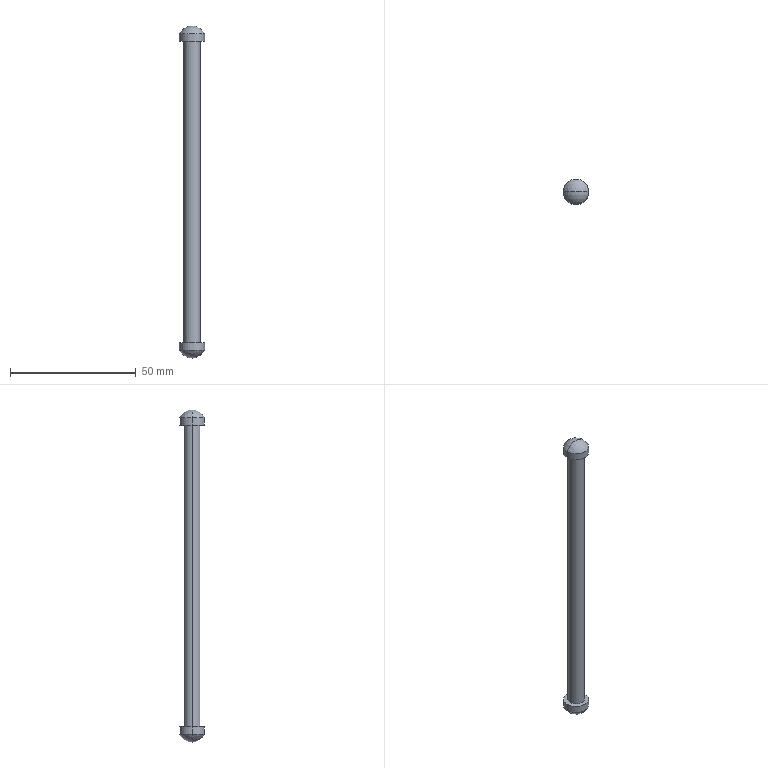Part | SolidWorks | features BaseBody 1 | 1 solid | 12 faces | box 10 x 10 x 132 mm | volume 4717 mm3 | cylinder 6 | sphere 4 | plane 2 | commonest cylinder face diameters 10 x4 6.5 x2
STEP:
#1=CARTESIAN_POINT('',(-30.,5.,-126.));
#2=VERTEX_POINT('',#1);
#3=CARTESIAN_POINT('',(-25.,5.,-123.));
#4=VERTEX_POINT('',#3);
#5=CARTESIAN_POINT('',(-30.,5.,-120.333));
#6=DIRECTION('',(0.,-1.,0.));
#7=DIRECTION('',(0.,0.,-1.));
#8=AXIS2_PLACEMENT_3D('',#5,#6,#7);
#9=CIRCLE('',#8,5.667);
#10=EDGE_CURVE('',#2,#4,#9,.T.);
#11=ORIENTED_EDGE('',*,*,#10,.F.);
#12=CARTESIAN_POINT('',(-35.,5.,-123.));
#13=VERTEX_POINT('',#12);
#14=CARTESIAN_POINT('',(-30.,5.,-120.333));
#15=DIRECTION('',(0.,1.,0.));
#16=DIRECTION('',(-1.,0.,0.));
#17=AXIS2_PLACEMENT_3D('',#14,#15,#16);
#18=CIRCLE('',#17,5.667);
#19=EDGE_CURVE('',#2,#13,#18,.T.);
#20=ORIENTED_EDGE('',*,*,#19,.T.);
#21=CARTESIAN_POINT('',(-30.,5.,-123.));
#22=DIRECTION('',(0.,0.,1.));
#23=DIRECTION('',(1.,0.,0.));
#24=AXIS2_PLACEMENT_3D('',#21,#22,#23);
#25=CIRCLE('',#24,5.);
#26=EDGE_CURVE('',#4,#13,#25,.T.);
#27=ORIENTED_EDGE('',*,*,#26,.F.);
#28=EDGE_LOOP('',(#11,#20,#27));
#29=FACE_OUTER_BOUND('',#28,.T.);
#30=CARTESIAN_POINT('',(-30.,5.,-120.333));
#31=DIRECTION('',(0.,1.,0.));
#32=DIRECTION('',(1.,0.,0.));
#33=AXIS2_PLACEMENT_3D('',#30,#31,#32);
#34=SPHERICAL_SURFACE('',#33,5.667);
#35=ADVANCED_FACE('',(#29),#34,.T.);
#36=ORIENTED_EDGE('',*,*,#26,.T.);
#37=CARTESIAN_POINT('',(-35.,5.,-120.));
#38=VERTEX_POINT('',#37);
#39=CARTESIAN_POINT('',(-35.,5.,-123.));
#40=DIRECTION('',(0.,0.,1.));
#41=VECTOR('',#40,1000.);
#42=LINE('',#39,#41);
#43=EDGE_CURVE('',#13,#38,#42,.T.);
#44=ORIENTED_EDGE('',*,*,#43,.T.);
#45=CARTESIAN_POINT('',(-25.,5.,-120.));
#46=VERTEX_POINT('',#45);
#47=CARTESIAN_POINT('',(-30.,5.,-120.));
#48=DIRECTION('',(0.,0.,1.));
#49=DIRECTION('',(1.,0.,0.));
#50=AXIS2_PLACEMENT_3D('',#47,#48,#49);
#51=CIRCLE('',#50,5.);
#52=EDGE_CURVE('',#46,#38,#51,.T.);
#53=ORIENTED_EDGE('',*,*,#52,.F.);
#54=CARTESIAN_POINT('',(-25.,5.,-123.));
#55=DIRECTION('',(0.,0.,1.));
#56=VECTOR('',#55,1000.);
#57=LINE('',#54,#56);
#58=EDGE_CURVE('',#4,#46,#57,.T.);
#59=ORIENTED_EDGE('',*,*,#58,.F.);
#60=EDGE_LOOP('',(#36,#44,#53,#59));
#61=FACE_OUTER_BOUND('',#60,.T.);
#62=CARTESIAN_POINT('',(-30.,5.,-123.));
#63=DIRECTION('',(0.,0.,1.));
#64=DIRECTION('',(1.,0.,0.));
#65=AXIS2_PLACEMENT_3D('',#62,#63,#64);
#66=CYLINDRICAL_SURFACE('',#65,5.);
#67=ADVANCED_FACE('',(#61),#66,.T.);
#68=CARTESIAN_POINT('',(-25.,5.,3.));
#69=VERTEX_POINT('',#68);
#70=CARTESIAN_POINT('',(-35.,5.,3.));
#71=VERTEX_POINT('',#70);
#72=CARTESIAN_POINT('',(-30.,5.,3.));
#73=DIRECTION('',(0.,0.,1.));
#74=DIRECTION('',(1.,0.,0.));
#75=AXIS2_PLACEMENT_3D('',#72,#73,#74);
#76=CIRCLE('',#75,5.);
#77=EDGE_CURVE('',#69,#71,#76,.T.);
#78=ORIENTED_EDGE('',*,*,#77,.T.);
#79=CARTESIAN_POINT('',(-30.,5.,6.));
#80=VERTEX_POINT('',#79);
#81=CARTESIAN_POINT('',(-30.,5.,0.3333));
#82=DIRECTION('',(0.,1.,0.));
#83=DIRECTION('',(-1.,0.,0.));
#84=AXIS2_PLACEMENT_3D('',#81,#82,#83);
#85=CIRCLE('',#84,5.667);
#86=EDGE_CURVE('',#71,#80,#85,.T.);
#87=ORIENTED_EDGE('',*,*,#86,.T.);
#88=CARTESIAN_POINT('',(-30.,5.,0.3333));
#89=DIRECTION('',(0.,-1.,0.));
#90=DIRECTION('',(0.,0.,-1.));
#91=AXIS2_PLACEMENT_3D('',#88,#89,#90);
#92=CIRCLE('',#91,5.667);
#93=EDGE_CURVE('',#69,#80,#92,.T.);
#94=ORIENTED_EDGE('',*,*,#93,.F.);
#95=EDGE_LOOP('',(#78,#87,#94));
#96=FACE_OUTER_BOUND('',#95,.T.);
#97=CARTESIAN_POINT('',(-30.,5.,0.3333));
#98=DIRECTION('',(0.,1.,0.));
#99=DIRECTION('',(1.,0.,0.));
#100=AXIS2_PLACEMENT_3D('',#97,#98,#99);
#101=SPHERICAL_SURFACE('',#100,5.667);
#102=ADVANCED_FACE('',(#96),#101,.T.);
#103=ORIENTED_EDGE('',*,*,#77,.F.);
#104=CARTESIAN_POINT('',(-25.,5.,0.));
#105=VERTEX_POINT('',#104);
#106=CARTESIAN_POINT('',(-25.,5.,3.));
#107=DIRECTION('',(0.,0.,-1.));
#108=VECTOR('',#107,1000.);
#109=LINE('',#106,#108);
#110=EDGE_CURVE('',#69,#105,#109,.T.);
#111=ORIENTED_EDGE('',*,*,#110,.T.);
#112=CARTESIAN_POINT('',(-35.,5.,0.));
#113=VERTEX_POINT('',#112);
#114=CARTESIAN_POINT('',(-30.,5.,0.));
#115=DIRECTION('',(0.,0.,1.));
#116=DIRECTION('',(1.,0.,0.));
#117=AXIS2_PLACEMENT_3D('',#114,#115,#116);
#118=CIRCLE('',#117,5.);
#119=EDGE_CURVE('',#105,#113,#118,.T.);
#120=ORIENTED_EDGE('',*,*,#119,.T.);
#121=CARTESIAN_POINT('',(-35.,5.,3.));
#122=DIRECTION('',(0.,0.,-1.));
#123=VECTOR('',#122,1000.);
#124=LINE('',#121,#123);
#125=EDGE_CURVE('',#71,#113,#124,.T.);
#126=ORIENTED_EDGE('',*,*,#125,.F.);
#127=EDGE_LOOP('',(#103,#111,#120,#126));
#128=FACE_OUTER_BOUND('',#127,.T.);
#129=CARTESIAN_POINT('',(-30.,5.,3.));
#130=DIRECTION('',(0.,0.,-1.));
#131=DIRECTION('',(-1.,0.,0.));
#132=AXIS2_PLACEMENT_3D('',#129,#130,#131);
#133=CYLINDRICAL_SURFACE('',#132,5.);
#134=ADVANCED_FACE('',(#128),#133,.T.);
#135=CARTESIAN_POINT('',(-26.75,5.,-120.));
#136=VERTEX_POINT('',#135);
#137=CARTESIAN_POINT('',(-33.25,5.,-120.));
#138=VERTEX_POINT('',#137);
#139=CARTESIAN_POINT('',(-30.,5.,-120.));
#140=DIRECTION('',(0.,0.,1.));
#141=DIRECTION('',(-1.,0.,0.));
#142=AXIS2_PLACEMENT_3D('',#139,#140,#141);
#143=CIRCLE('',#142,3.25);
#144=EDGE_CURVE('',#136,#138,#143,.T.);
#145=ORIENTED_EDGE('',*,*,#144,.T.);
#146=CARTESIAN_POINT('',(-33.25,5.,0.));
#147=VERTEX_POINT('',#146);
#148=CARTESIAN_POINT('',(-33.25,5.,-120.));
#149=DIRECTION('',(0.,0.,1.));
#150=VECTOR('',#149,1000.);
#151=LINE('',#148,#150);
#152=EDGE_CURVE('',#138,#147,#151,.T.);
#153=ORIENTED_EDGE('',*,*,#152,.T.);
#154=CARTESIAN_POINT('',(-26.75,5.,0.));
#155=VERTEX_POINT('',#154);
#156=CARTESIAN_POINT('',(-30.,5.,0.));
#157=DIRECTION('',(0.,0.,1.));
#158=DIRECTION('',(1.,0.,0.));
#159=AXIS2_PLACEMENT_3D('',#156,#157,#158);
#160=CIRCLE('',#159,3.25);
#161=EDGE_CURVE('',#155,#147,#160,.T.);
#162=ORIENTED_EDGE('',*,*,#161,.F.);
#163=CARTESIAN_POINT('',(-26.75,5.,-120.));
#164=DIRECTION('',(0.,0.,1.));
#165=VECTOR('',#164,1000.);
#166=LINE('',#163,#165);
#167=EDGE_CURVE('',#136,#155,#166,.T.);
#168=ORIENTED_EDGE('',*,*,#167,.F.);
#169=EDGE_LOOP('',(#145,#153,#162,#168));
#170=FACE_OUTER_BOUND('',#169,.T.);
#171=CARTESIAN_POINT('',(-30.,5.,-120.));
#172=DIRECTION('',(0.,0.,1.));
#173=DIRECTION('',(1.,0.,0.));
#174=AXIS2_PLACEMENT_3D('',#171,#172,#173);
#175=CYLINDRICAL_SURFACE('',#174,3.25);
#176=ADVANCED_FACE('',(#170),#175,.T.);
#177=ORIENTED_EDGE('',*,*,#152,.F.);
#178=CARTESIAN_POINT('',(-30.,5.,-120.));
#179=DIRECTION('',(0.,0.,1.));
#180=DIRECTION('',(-1.,0.,0.));
#181=AXIS2_PLACEMENT_3D('',#178,#179,#180);
#182=CIRCLE('',#181,3.25);
#183=EDGE_CURVE('',#138,#136,#182,.T.);
#184=ORIENTED_EDGE('',*,*,#183,.T.);
#185=ORIENTED_EDGE('',*,*,#167,.T.);
#186=CARTESIAN_POINT('',(-30.,5.,0.));
#187=DIRECTION('',(0.,0.,1.));
#188=DIRECTION('',(1.,0.,0.));
#189=AXIS2_PLACEMENT_3D('',#186,#187,#188);
#190=CIRCLE('',#189,3.25);
#191=EDGE_CURVE('',#147,#155,#190,.T.);
#192=ORIENTED_EDGE('',*,*,#191,.F.);
#193=EDGE_LOOP('',(#177,#184,#185,#192));
#194=FACE_OUTER_BOUND('',#193,.T.);
#195=CARTESIAN_POINT('',(-30.,5.,-120.));
#196=DIRECTION('',(0.,0.,1.));
#197=DIRECTION('',(1.,0.,0.));
#198=AXIS2_PLACEMENT_3D('',#195,#196,#197);
#199=CYLINDRICAL_SURFACE('',#198,3.25);
#200=ADVANCED_FACE('',(#194),#199,.T.);
#201=ORIENTED_EDGE('',*,*,#110,.F.);
#202=CARTESIAN_POINT('',(-30.,5.,3.));
#203=DIRECTION('',(0.,0.,1.));
#204=DIRECTION('',(1.,0.,0.));
#205=AXIS2_PLACEMENT_3D('',#202,#203,#204);
#206=CIRCLE('',#205,5.);
#207=EDGE_CURVE('',#71,#69,#206,.T.);
#208=ORIENTED_EDGE('',*,*,#207,.F.);
#209=ORIENTED_EDGE('',*,*,#125,.T.);
#210=CARTESIAN_POINT('',(-30.,5.,0.));
#211=DIRECTION('',(0.,0.,1.));
#212=DIRECTION('',(1.,0.,0.));
#213=AXIS2_PLACEMENT_3D('',#210,#211,#212);
#214=CIRCLE('',#213,5.);
#215=EDGE_CURVE('',#113,#105,#214,.T.);
#216=ORIENTED_EDGE('',*,*,#215,.T.);
#217=EDGE_LOOP('',(#201,#208,#209,#216));
#218=FACE_OUTER_BOUND('',#217,.T.);
#219=CARTESIAN_POINT('',(-30.,5.,3.));
#220=DIRECTION('',(0.,0.,-1.));
#221=DIRECTION('',(-1.,0.,0.));
#222=AXIS2_PLACEMENT_3D('',#219,#220,#221);
#223=CYLINDRICAL_SURFACE('',#222,5.);
#224=ADVANCED_FACE('',(#218),#223,.T.);
#225=ORIENTED_EDGE('',*,*,#86,.F.);
#226=ORIENTED_EDGE('',*,*,#207,.T.);
#227=ORIENTED_EDGE('',*,*,#93,.T.);
#228=EDGE_LOOP('',(#225,#226,#227));
#229=FACE_OUTER_BOUND('',#228,.T.);
#230=CARTESIAN_POINT('',(-30.,5.,0.3333));
#231=DIRECTION('',(0.,1.,0.));
#232=DIRECTION('',(1.,0.,0.));
#233=AXIS2_PLACEMENT_3D('',#230,#231,#232);
#234=SPHERICAL_SURFACE('',#233,5.667);
#235=ADVANCED_FACE('',(#229),#234,.T.);
#236=ORIENTED_EDGE('',*,*,#161,.T.);
#237=ORIENTED_EDGE('',*,*,#191,.T.);
#238=EDGE_LOOP('',(#236,#237));
#239=FACE_BOUND('',#238,.T.);
#240=ORIENTED_EDGE('',*,*,#215,.F.);
#241=ORIENTED_EDGE('',*,*,#119,.F.);
#242=EDGE_LOOP('',(#240,#241));
#243=FACE_OUTER_BOUND('',#242,.T.);
#244=CARTESIAN_POINT('',(-30.,5.,0.));
#245=DIRECTION('',(0.,0.,1.));
#246=DIRECTION('',(1.,0.,0.));
#247=AXIS2_PLACEMENT_3D('',#244,#245,#246);
#248=PLANE('',#247);
#249=ADVANCED_FACE('',(#239,#243),#248,.F.);
#250=ORIENTED_EDGE('',*,*,#43,.F.);
#251=CARTESIAN_POINT('',(-30.,5.,-123.));
#252=DIRECTION('',(0.,0.,1.));
#253=DIRECTION('',(1.,0.,0.));
#254=AXIS2_PLACEMENT_3D('',#251,#252,#253);
#255=CIRCLE('',#254,5.);
#256=EDGE_CURVE('',#13,#4,#255,.T.);
#257=ORIENTED_EDGE('',*,*,#256,.T.);
#258=ORIENTED_EDGE('',*,*,#58,.T.);
#259=CARTESIAN_POINT('',(-30.,5.,-120.));
#260=DIRECTION('',(0.,0.,1.));
#261=DIRECTION('',(1.,0.,0.));
#262=AXIS2_PLACEMENT_3D('',#259,#260,#261);
#263=CIRCLE('',#262,5.);
#264=EDGE_CURVE('',#38,#46,#263,.T.);
#265=ORIENTED_EDGE('',*,*,#264,.F.);
#266=EDGE_LOOP('',(#250,#257,#258,#265));
#267=FACE_OUTER_BOUND('',#266,.T.);
#268=CARTESIAN_POINT('',(-30.,5.,-123.));
#269=DIRECTION('',(0.,0.,1.));
#270=DIRECTION('',(1.,0.,0.));
#271=AXIS2_PLACEMENT_3D('',#268,#269,#270);
#272=CYLINDRICAL_SURFACE('',#271,5.);
#273=ADVANCED_FACE('',(#267),#272,.T.);
#274=ORIENTED_EDGE('',*,*,#19,.F.);
#275=ORIENTED_EDGE('',*,*,#10,.T.);
#276=ORIENTED_EDGE('',*,*,#256,.F.);
#277=EDGE_LOOP('',(#274,#275,#276));
#278=FACE_OUTER_BOUND('',#277,.T.);
#279=CARTESIAN_POINT('',(-30.,5.,-120.333));
#280=DIRECTION('',(0.,1.,0.));
#281=DIRECTION('',(1.,0.,0.));
#282=AXIS2_PLACEMENT_3D('',#279,#280,#281);
#283=SPHERICAL_SURFACE('',#282,5.667);
#284=ADVANCED_FACE('',(#278),#283,.T.);
#285=ORIENTED_EDGE('',*,*,#144,.F.);
#286=ORIENTED_EDGE('',*,*,#183,.F.);
#287=EDGE_LOOP('',(#285,#286));
#288=FACE_BOUND('',#287,.T.);
#289=ORIENTED_EDGE('',*,*,#52,.T.);
#290=ORIENTED_EDGE('',*,*,#264,.T.);
#291=EDGE_LOOP('',(#289,#290));
#292=FACE_OUTER_BOUND('',#291,.T.);
#293=CARTESIAN_POINT('',(-30.,5.,-120.));
#294=DIRECTION('',(0.,0.,-1.));
#295=DIRECTION('',(1.,0.,0.));
#296=AXIS2_PLACEMENT_3D('',#293,#294,#295);
#297=PLANE('',#296);
#298=ADVANCED_FACE('',(#288,#292),#297,.F.);
#299=CLOSED_SHELL('',(#35,#67,#102,#134,#176,#200,#224,#235,#249,#273,#284,#298));
#300=MANIFOLD_SOLID_BREP('',#299);
#301=CARTESIAN_POINT('',(0.,0.,0.));
#302=DIRECTION('',(0.,0.,1.));
#303=DIRECTION('',(1.,0.,0.));
#304=AXIS2_PLACEMENT_3D('',#301,#302,#303);
#305=(LENGTH_UNIT()NAMED_UNIT(*)SI_UNIT(.MILLI.,.METRE.));
#306=UNCERTAINTY_MEASURE_WITH_UNIT(LENGTH_MEASURE(0.00001),#305,'','');
#307=(NAMED_UNIT(*)PLANE_ANGLE_UNIT()SI_UNIT($,.RADIAN.));
#308=(NAMED_UNIT(*)SI_UNIT($,.STERADIAN.)SOLID_ANGLE_UNIT());
#309=(GEOMETRIC_REPRESENTATION_CONTEXT(3)GLOBAL_UNCERTAINTY_ASSIGNED_CONTEXT((#306))GLOBAL_UNIT_ASSIGNED_CONTEXT((#305,#307,#308))REPRESENTATION_CONTEXT('',''));
#310=ADVANCED_BREP_SHAPE_REPRESENTATION('',(#300,#304),#309);